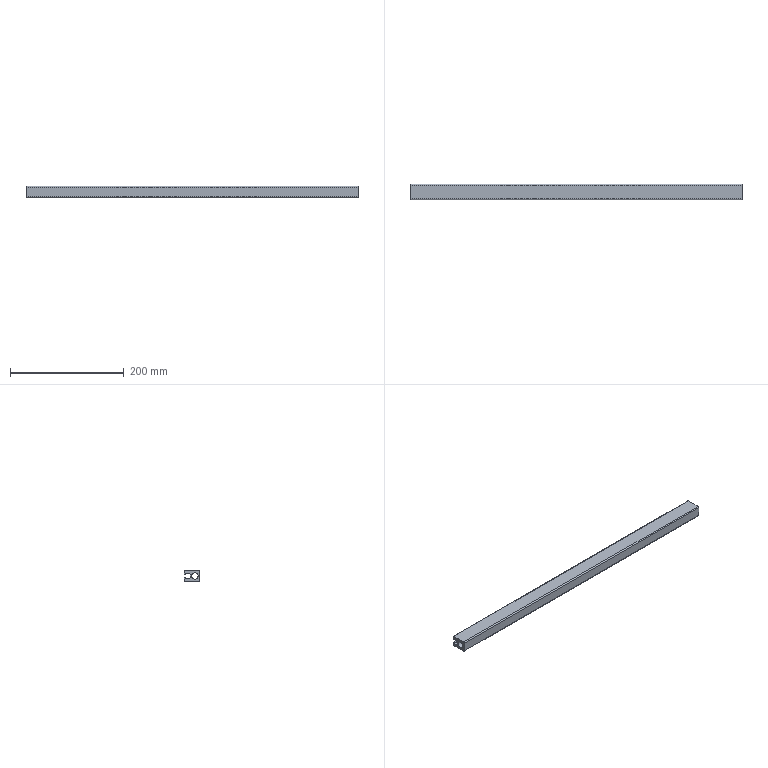Part | SolidWorks | features HoleWzd 7, Extrusion 1, Fillet 1, ICE 1 | 1 solid | 49 faces | box 585 x 28 x 20 mm | volume 202510 mm3 | cylinder 29 | plane 13 | cone 7 | commonest cylinder face diameters 4.2 x16 11.8 x6 4 x4 11.5 x2 22.589 x1